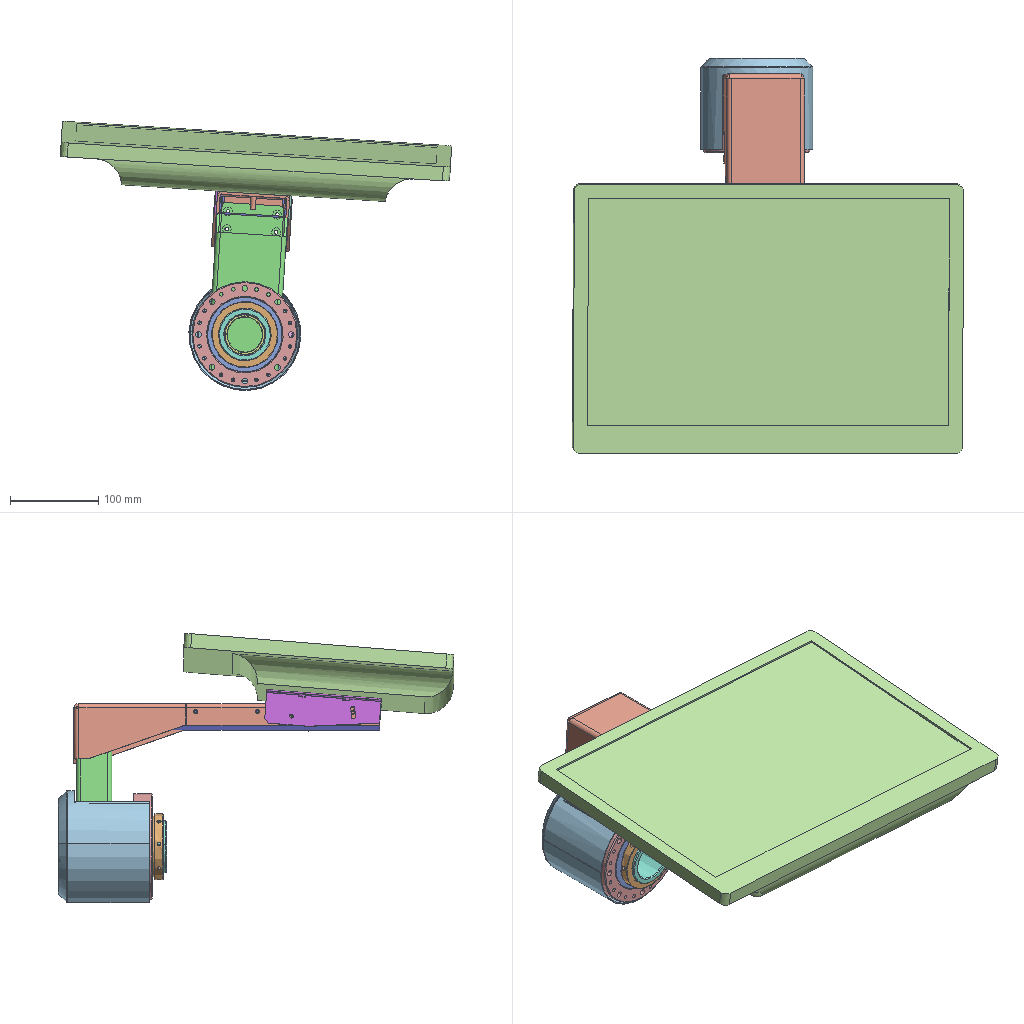Assembly | SolidWorks | 17 different items | 22 placed | box 444 x 449 x 305 mm
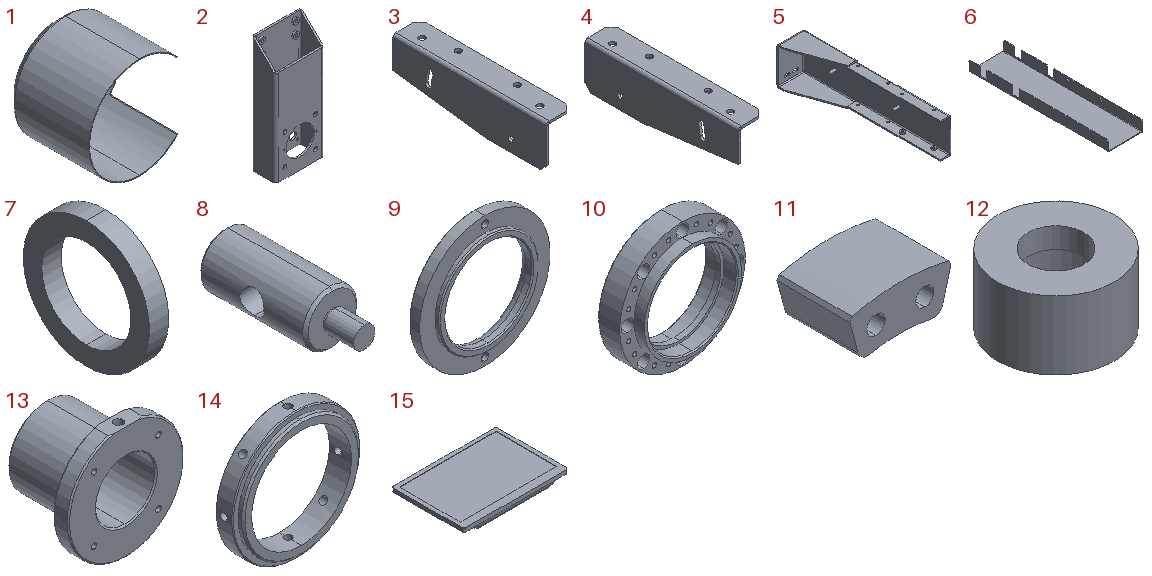Parts list (item | name | quantity | size | volume | features):
1 | - | x1 | 127 x 103.5 x 127 mm | 43057 mm3 | features Fillet 2, Chamfer 1, Extrusion 1, HoleWzd 1, ICE 1, Shell 1
2 | - | x1 | 80 x 40 x 190 mm | 108540 mm3 | features HoleWzd 5, ICE 4, Extrusion 1
3 | - | x1 | 22.5 x 130 x 37 mm | 13846 mm3 | features ICE 3, Chamfer 2, Cut 2, FlatPattern 1, HoleWzd 1, SMBaseFlange 1, SheetMetal 1
4 | - | x1 | 22.5 x 130 x 37 mm | 13846 mm3 | features ICE 3, Chamfer 2, Cut 2, FlatPattern 1, HoleWzd 1, SMBaseFlange 1, SheetMetal 1
5 | - | x1 | 63 x 346.5 x 88 mm | 160179 mm3 | features ICE 7, HoleWzd 5, Chamfer 2, EdgeFlange 2, Cut 1, FlatPattern 1, SMBaseFlange 1, SheetMetal 1
6 | - | x1 | 75.5 x 298.5 x 21.5 mm | 49860 mm3 | features Chamfer 1, Cut 1, EdgeFlange 1, FlatPattern 1, HoleWzd 1, ICE 1, MirrorPattern 1, SMBaseFlange 1, SheetMetal 1
7 | - | x2 | 13 x 85 x 85 mm | 37012 mm3 | features Extrusion 1
8 | - | x4 | 10 x 26 x 10 mm | 1414 mm3 | features ICE 2, Chamfer 1, Extrusion 1, HoleWzd 1, RevCut 1
9 | - | x1 | 60 x 7 x 60 mm | 7951 mm3 | features Chamfer 1, Extrusion 1, Fillet 1, HoleWzd 1, ICE 1
10 | - | x1 | 120 x 31 x 120 mm | 115684 mm3 | features CirPattern 3, Chamfer 2, Cut 2, HoleWzd 2, ICE 2, Extrusion 1
11 | - | x2 | 30.541 x 22 x 14.401 mm | 6316 mm3 | features Chamfer 1, Extrusion 1, Fillet 1, HoleWzd 1, ICE 1
12 | - | x1 | 17 x 17 x 10 mm | 1256 mm3 | features Cut 1, Extrusion 1
13 | - | x1 | 90 x 62 x 88 mm | 114650 mm3 | features ICE 4, HoleWzd 2, Chamfer 1, Extrusion 1
14 | - | x1 | 75 x 13 x 75 mm | 19213 mm3 | features Chamfer 2, CirPattern 1, Extrusion 1, HoleWzd 1, ICE 1
15 | - | x1 | 442 x 306 x 46 mm | 4020857 mm3 | features Fillet 3, ICE 2, Extrusion 1, HoleWzd 1
16 | hexagon socket head cap screws gb | x1 | - | - | -
17 | plain washers-n series-grade a gb | x1 | - | - | -
Mates (type | each side: item.copy, entity, surface, feature):
Coincident | 8.1 face plane Boss-Extrude 1 | 2.1 face plane Boss-Extrude 1
Concentric | 8.1 face cylinder Boss-Extrude 1 | 2.1 face cylinder M4 Tapped Hole 1
Concentric | 8.2 face cylinder Boss-Extrude 1 | 2.1 face cylinder M4 Tapped Hole 1
Concentric | 8.3 face cylinder Boss-Extrude 1 | 2.1 face cylinder M4 Tapped Hole 1
Concentric | 8.4 face cylinder Boss-Extrude 1 | 2.1 face cylinder M4 Tapped Hole 1
Coincident | 2.1 face plane Boss-Extrude 1 | 9.1 face plane Cut-Extrude 1
Concentric | 2.1 face cylinder Cut-Extrude 1 | 9.1 face cylinder Boss-Extrude 1
Concentric | 2.1 face cylinder M3 Tapped Hole 1 | 9.1 face cylinder Hole size per socket head cap screw type 1
Coincident | 2.1 face plane Boss-Extrude 1 | 5.1 face plane Base-Flange 1
DistanceDim | 2.1 face plane Boss-Extrude 1 | 5.1 face plane Edge-Flange 1
DistanceDim | 5.1 face plane Edge-Flange 1 | 2.1 face plane Boss-Extrude 1
Coincident | 8.2 face plane Boss-Extrude 1 | 8.1 face plane Boss-Extrude 1
Concentric | 8.2 face cylinder M4 Tapped Hole 1 | 1.1 face cylinder Ø4.5 (4.5) DiameterHole 1
Coincident | 8.1 face plane Boss-Extrude 1 | 8.3 face plane Boss-Extrude 1
Coincident | 8.1 face plane Boss-Extrude 1 | 8.4 face plane Boss-Extrude 1
Coincident | 8.4 face plane Boss-Extrude 1 | 1.1 face plane Shell1
Concentric | 8.4 face cylinder M4 Tapped Hole 1 | 1.1 face cylinder Ø4.5 (4.5) DiameterHole 1
Concentric | 3.1 face cylinder Cut-Extrude 1 | 15.1 face cylinder M4 Tapped Hole 1
Coincident | 5.1 face plane Edge-Flange 2 | 3.1 face plane Base-Flange 1
Concentric | 5.1 face cylinder Ø5.0 (5) DiameterHole 2 | 3.1 face cylinder Cut-Extrude 2
Parallel | 4.1 face plane Base-Flange 1 | 3.1 face plane Base-Flange 1
Coincident | 4.1 face plane Base-Flange 1 | 15.1 face plane Boss-Extrude 2
Concentric | 4.1 face cylinder Cut-Extrude 1 | 15.1 face cylinder M4 Tapped Hole 1
Coincident | 5.1 face plane Edge-Flange 2 | 4.1 face plane Base-Flange 1
Concentric | 5.1 face cylinder Ø5.0 (5) DiameterHole 1 | 4.1 face cylinder Cut-Extrude 2
Coincident | 5.1 face plane Edge-Flange 2 | 6.1 face plane Base-Flange 1 | 2 times
Coincident | 5.1 face plane Edge-Flange 2 | 6.1 face plane Edge-Flange 1
Coincident | 10.1 face plane Cut-Extrude 2 | 7.1 face plane Boss-Extrude 1
Concentric | 10.1 face cylinder Cut-Extrude 2 | 7.1 face cylinder Boss-Extrude 1
Coincident | 10.1 face plane Cut-Extrude 3 | 7.2 face plane Boss-Extrude 1
Concentric | 10.1 face cylinder Boss-Extrude 1 | 11.1 face cylinder Boss-Extrude 1
Coincident | 10.1 face plane Cut-Extrude 4 | 11.1 face plane Boss-Extrude 1
Concentric | 10.1 face cylinder Boss-Extrude 1 | 11.2 face cylinder Boss-Extrude 1
Coincident | 10.1 face plane Cut-Extrude 4 | 11.2 face plane Boss-Extrude 1
Concentric | 10.1 face cylinder CirPattern 1 | 11.2 face cylinder Hole size per socket head cap screw type 1
Concentric | 10.1 face cylinder CirPattern 1 | 11.1 face cylinder Hole size per socket head cap screw type 1
Coincident | 7.2 face plane Boss-Extrude 1 | 13.1 face plane Boss-Extrude 3
Coincident | 13.1 face plane Cut-Extrude 2 | 12.1 face plane Boss-Extrude 1
Concentric | 12.1 face cylinder Boss-Extrude 1 | 13.1 face cylinder M8 Tapped Hole 1
Concentric | 13.1 face cylinder Boss-Extrude 2 | 14.1 face cylinder Boss-Extrude 1
Coincident | 13.1 face plane Boss-Extrude 1 | 2.1 face plane Boss-Extrude 1
Concentric | 13.1 face cylinder M5 Tapped Hole 1 | 2.1 face cylinder Ø6.5 (6.5) DiameterHole 1
Concentric | 13.1 face cylinder Cut-Extrude 1 | 9.1 face cylinder Boss-Extrude 1